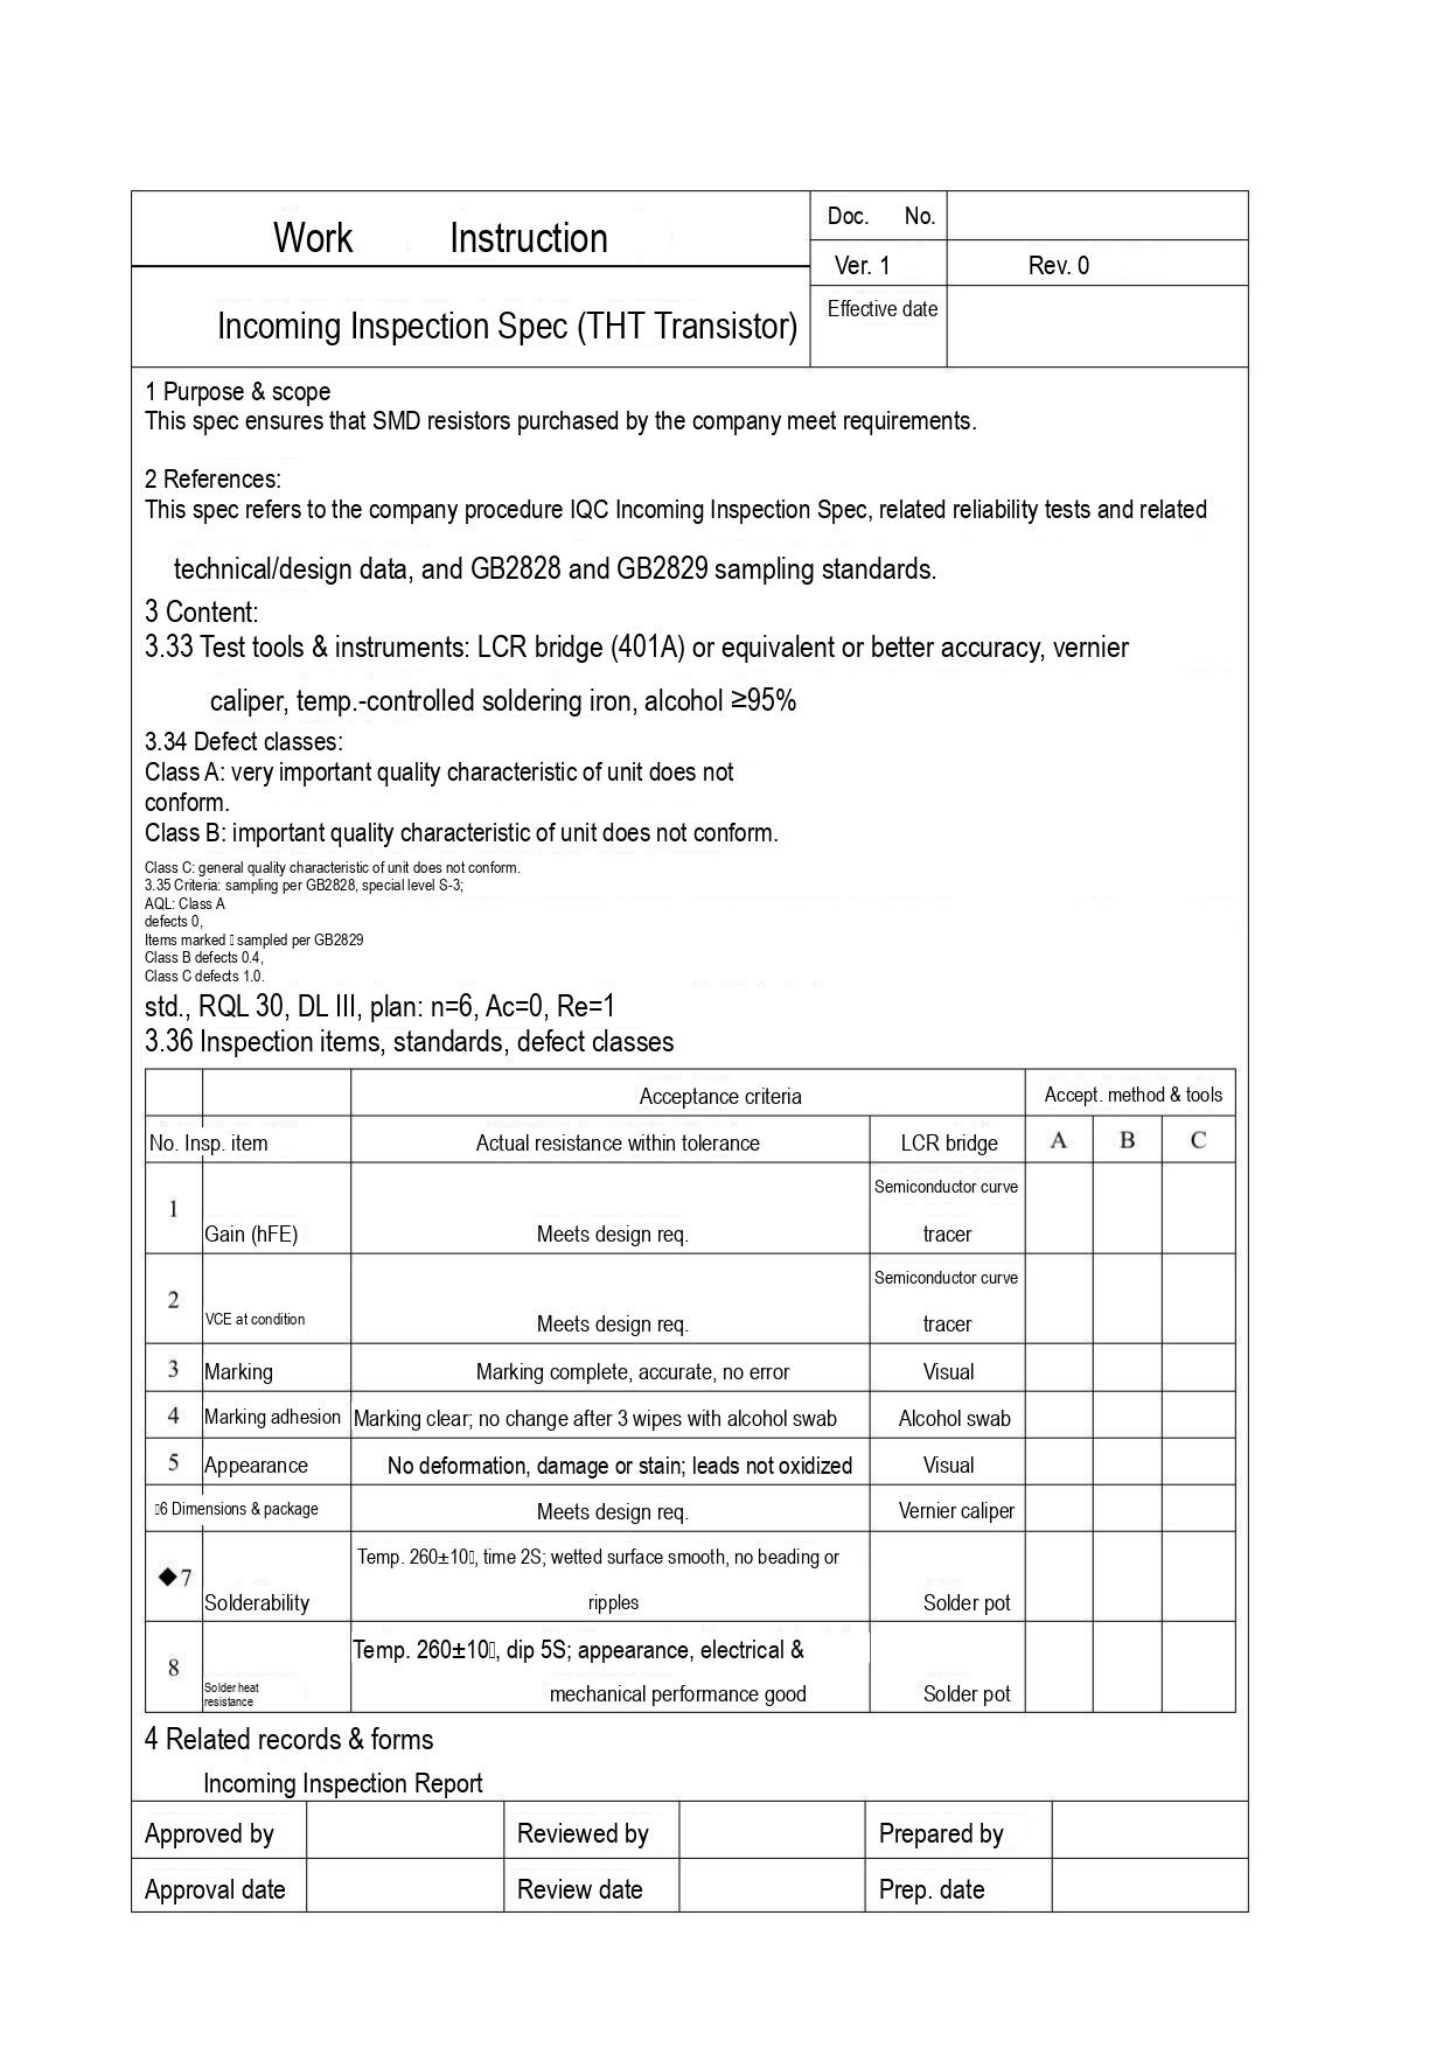| Work Instruction | Doc. No. | |
|---|---|---|
| | Ver. 1 | Rev. 0 |
| Incoming Inspection Spec (THT Transistor) | Effective date | |

1 Purpose & scope
This spec ensures that SMD resistors purchased by the company meet requirements.

2 References:
This spec refers to the company procedure IQC Incoming Inspection Spec, related reliability tests and related technical/design data, and GB2828 and GB2829 sampling standards.

3 Content:
3.33 Test tools & instruments: LCR bridge (401A) or equivalent or better accuracy, vernier caliper, temp.-controlled soldering iron, alcohol ≥95%
3.34 Defect classes:
Class A: very important quality characteristic of unit does not conform.
Class B: important quality characteristic of unit does not conform.
Class C: general quality characteristic of unit does not conform.
3.35 Criteria: sampling per GB2828, special level S-3;
AQL: Class A
defects 0,
Items marked □ sampled per GB2829
Class B defects 0.4,
Class C defects 1.0.
std., RQL 30, DL III, plan: n=6, Ac=0, Re=1
3.36 Inspection items, standards, defect classes

| | | Acceptance criteria | | Accept. method & tools | | |
|---|---|---|---|---|---|---|
| No. | Insp. item | Actual resistance within tolerance | LCR bridge | A | B | C |
| 1 | Gain (hFE) | Meets design req. | Semiconductor curve tracer | | | |
| 2 | VCE at condition | Meets design req. | Semiconductor curve tracer | | | |
| 3 | Marking | Marking complete, accurate, no error | Visual | | | |
| 4 | Marking adhesion | Marking clear; no change after 3 wipes with alcohol swab | Alcohol swab | | | |
| 5 | Appearance | No deformation, damage or stain; leads not oxidized | Visual | | | |
| □6 | Dimensions & package | Meets design req. | Vernier caliper | | | |
| ◆7 | Solderability | Temp. 260±10□, time 2S; wetted surface smooth, no beading or ripples | Solder pot | | | |
| 8 | Solder heat resistance | Temp. 260±10□, dip 5S; appearance, electrical & mechanical performance good | Solder pot | | | |

4 Related records & forms
Incoming Inspection Report

| Approved by | | Reviewed by | | Prepared by | |
|---|---|---|---|---|---|
| Approval date | | Review date | | Prep. date | |
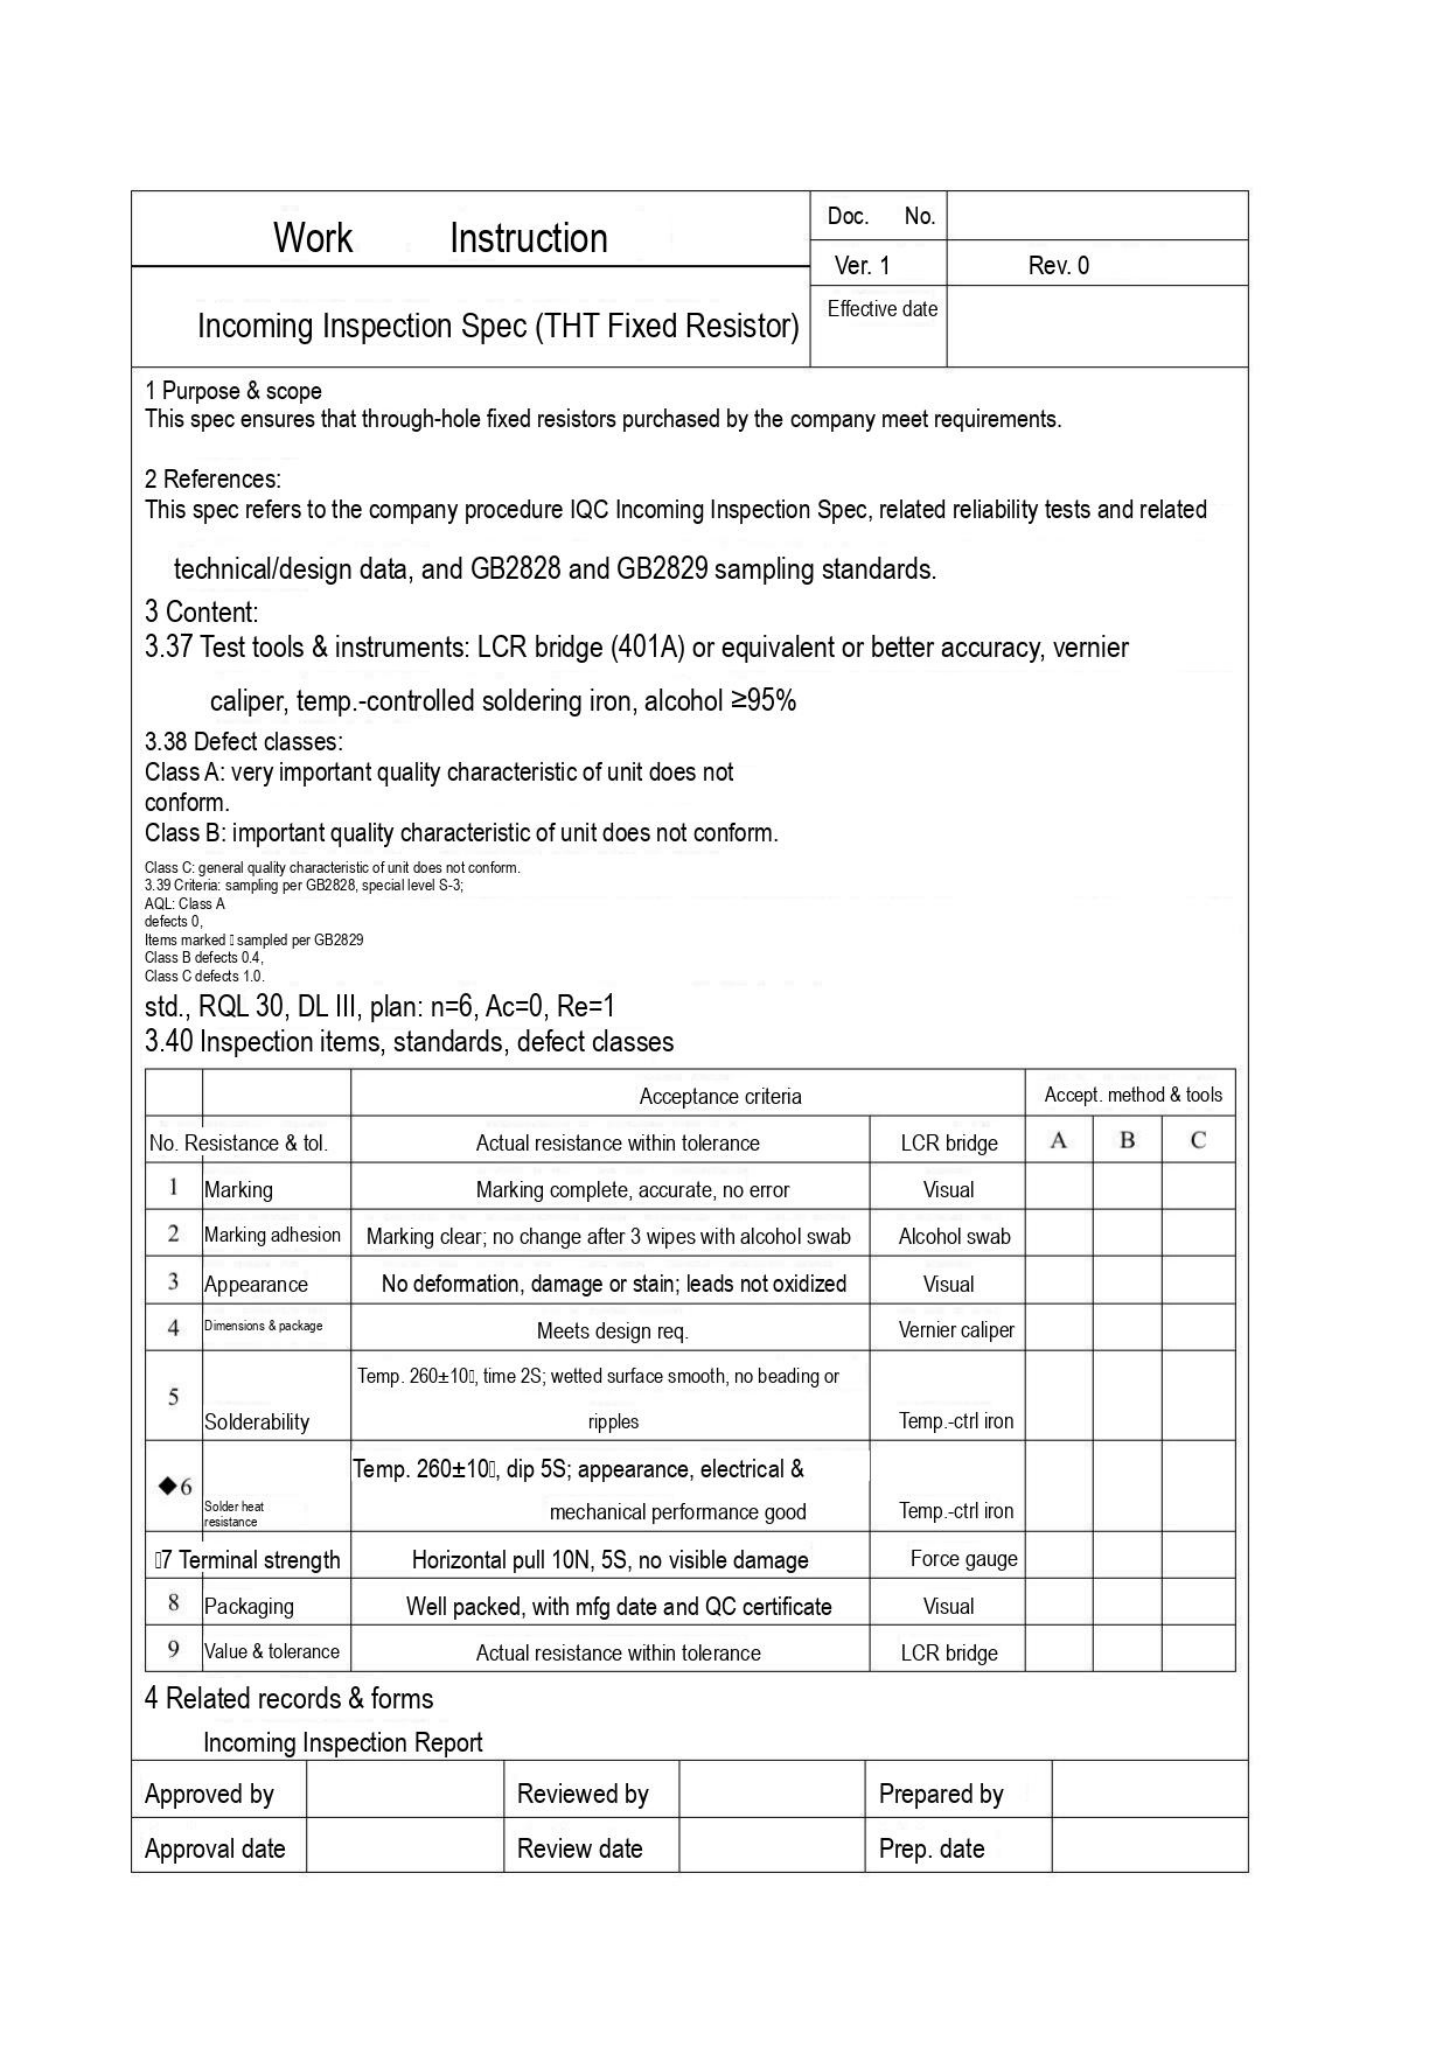| Work Instruction | Doc. No. | |
|---|---|---|
| | Ver. 1 | Rev. 0 |
| Incoming Inspection Spec (THT Fixed Resistor) | Effective date | |

1 Purpose & scope
This spec ensures that through-hole fixed resistors purchased by the company meet requirements.

2 References:
This spec refers to the company procedure IQC Incoming Inspection Spec, related reliability tests and related technical/design data, and GB2828 and GB2829 sampling standards.

3 Content:
3.37 Test tools & instruments: LCR bridge (401A) or equivalent or better accuracy, vernier caliper, temp.-controlled soldering iron, alcohol ≥95%
3.38 Defect classes:
Class A: very important quality characteristic of unit does not conform.
Class B: important quality characteristic of unit does not conform.
Class C: general quality characteristic of unit does not conform.
3.39 Criteria: sampling per GB2828, special level S-3;
AQL: Class A defects 0,
Items marked □ sampled per GB2829
Class B defects 0.4,
Class C defects 1.0.
std., RQL 30, DL III, plan: n=6, Ac=0, Re=1
3.40 Inspection items, standards, defect classes

| | | Acceptance criteria | | Accept. method & tools | | |
|---|---|---|---|---|---|---|
| No. | Resistance & tol. | Actual resistance within tolerance | LCR bridge | A | B | C |
| 1 | Marking | Marking complete, accurate, no error | Visual | | | |
| 2 | Marking adhesion | Marking clear; no change after 3 wipes with alcohol swab | Alcohol swab | | | |
| 3 | Appearance | No deformation, damage or stain; leads not oxidized | Visual | | | |
| 4 | Dimensions & package | Meets design req. | Vernier caliper | | | |
| 5 | Solderability | Temp. 260±10□, time 2S; wetted surface smooth, no beading or ripples | Temp.-ctrl iron | | | |
| ◆6 | Solder heat resistance | Temp. 260±10□, dip 5S; appearance, electrical & mechanical performance good | Temp.-ctrl iron | | | |
| □7 | Terminal strength | Horizontal pull 10N, 5S, no visible damage | Force gauge | | | |
| 8 | Packaging | Well packed, with mfg date and QC certificate | Visual | | | |
| 9 | Value & tolerance | Actual resistance within tolerance | LCR bridge | | | |

4 Related records & forms
Incoming Inspection Report

| Approved by | | Reviewed by | | Prepared by | |
|---|---|---|---|---|---|
| Approval date | | Review date | | Prep. date | |
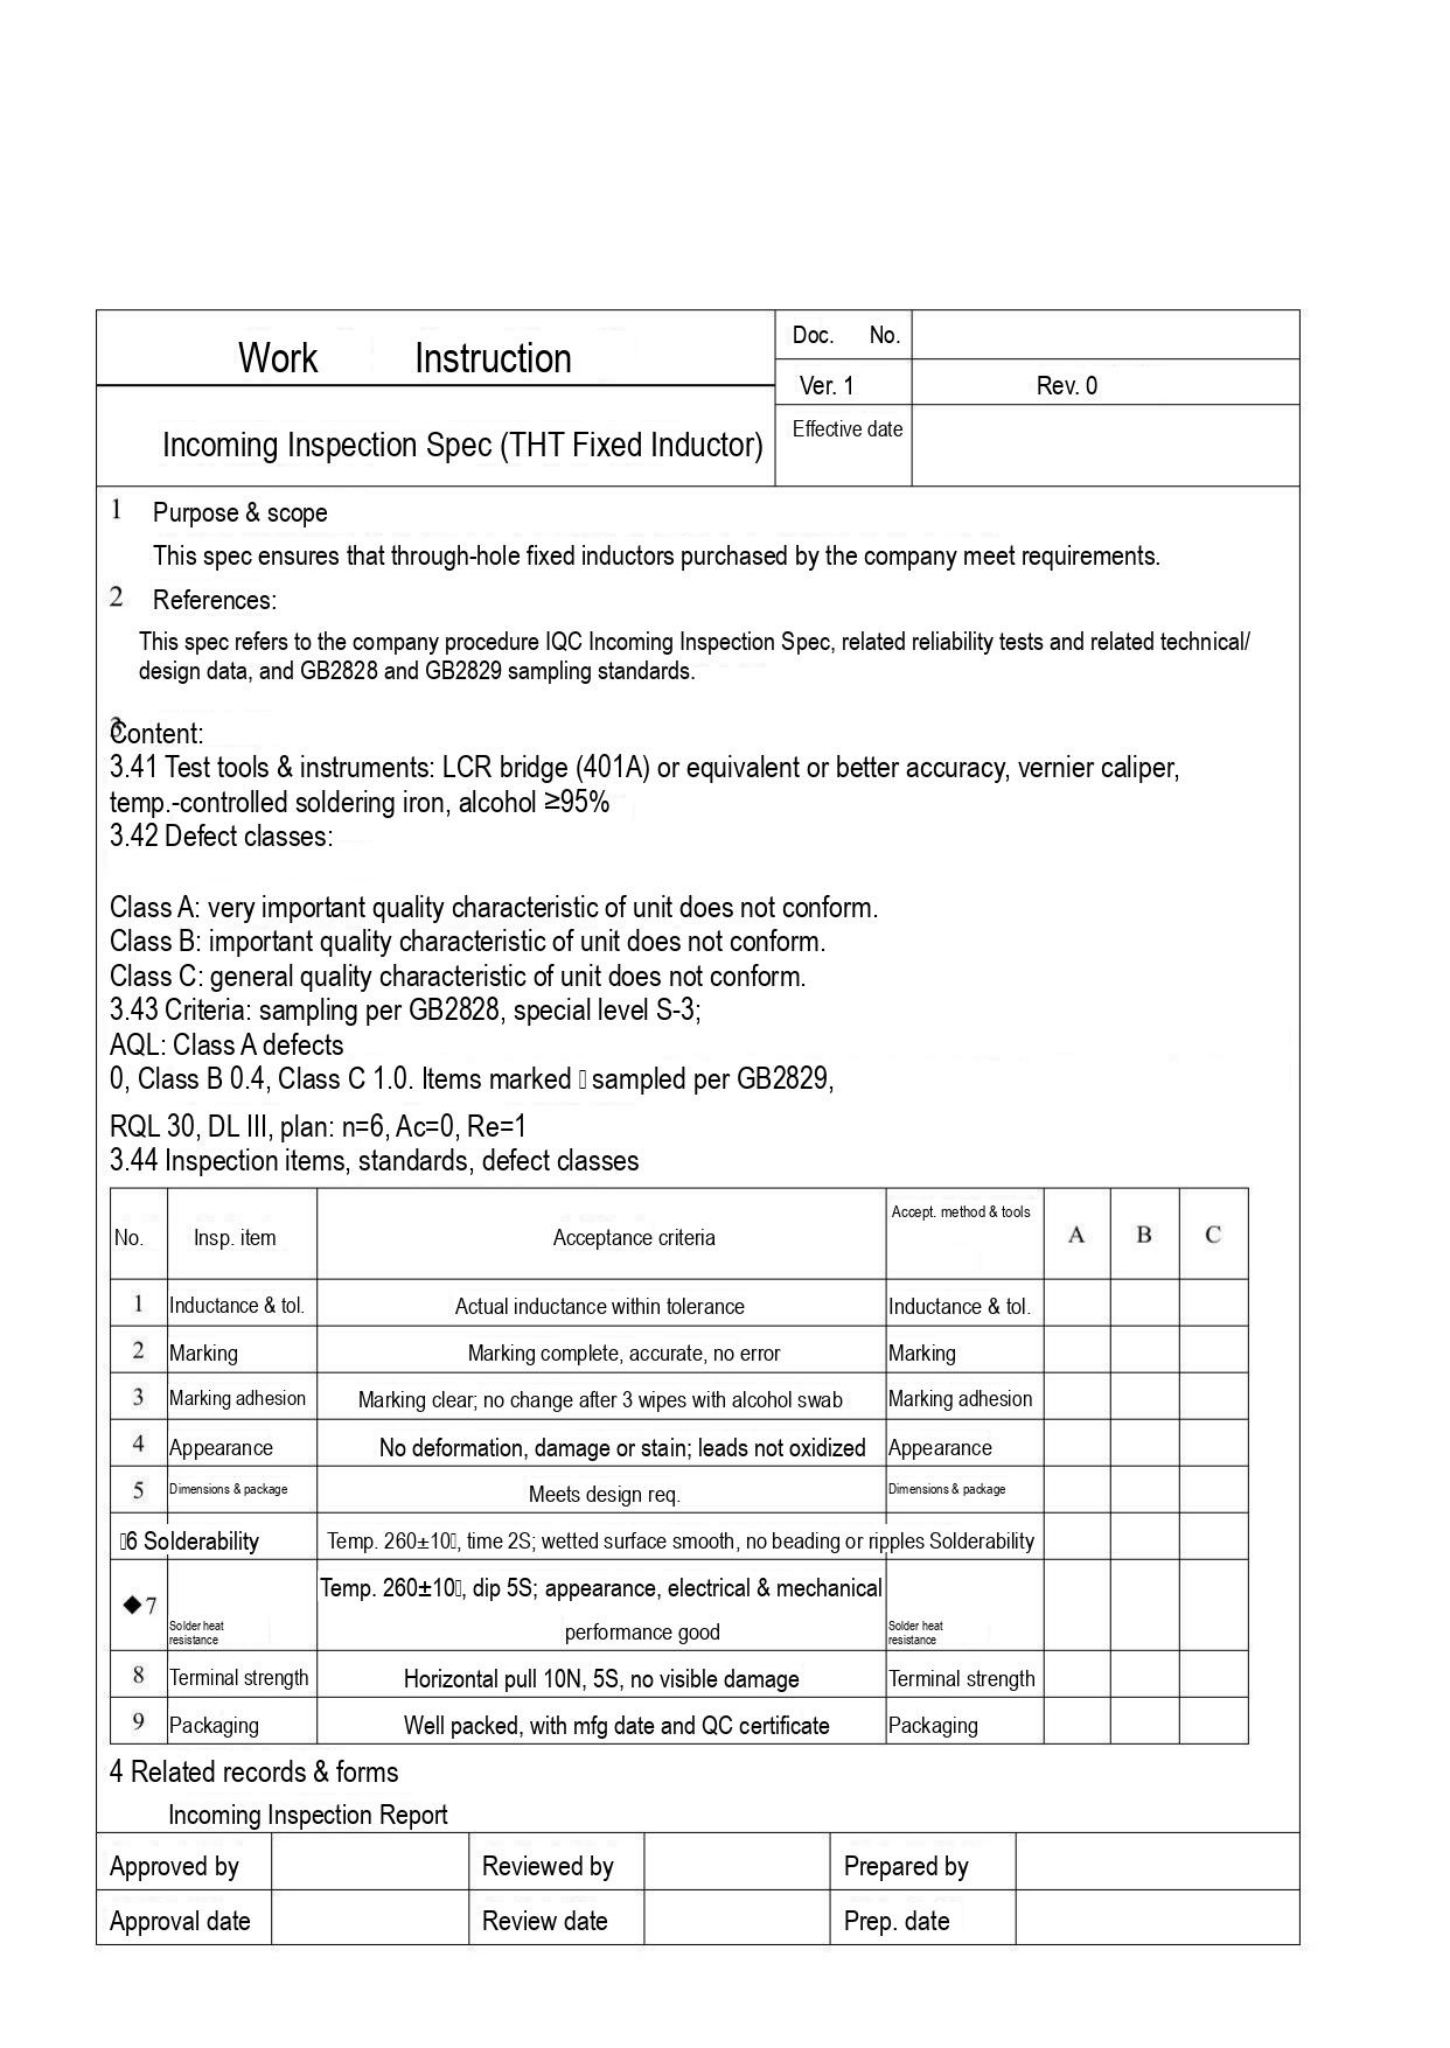# Work Instruction

| Work Instruction | Doc. No. | |
|---|---|---|
| | Ver. 1 | Rev. 0 |
| Incoming Inspection Spec (THT Fixed Inductor) | Effective date | |

1 Purpose & scope

This spec ensures that through-hole fixed inductors purchased by the company meet requirements.

2 References:

This spec refers to the company procedure IQC Incoming Inspection Spec, related reliability tests and related technical/ design data, and GB2828 and GB2829 sampling standards.

3 Content:

3.41 Test tools & instruments: LCR bridge (401A) or equivalent or better accuracy, vernier caliper, temp.-controlled soldering iron, alcohol ≥95%

3.42 Defect classes:

Class A: very important quality characteristic of unit does not conform.
Class B: important quality characteristic of unit does not conform.
Class C: general quality characteristic of unit does not conform.

3.43 Criteria: sampling per GB2828, special level S-3;
AQL: Class A defects
0, Class B 0.4, Class C 1.0. Items marked □ sampled per GB2829,

RQL 30, DL III, plan: n=6, Ac=0, Re=1

3.44 Inspection items, standards, defect classes

| No. | Insp. item | Acceptance criteria | Accept. method & tools | A | B | C |
|---|---|---|---|---|---|---|
| 1 | Inductance & tol. | Actual inductance within tolerance | Inductance & tol. | | | |
| 2 | Marking | Marking complete, accurate, no error | Marking | | | |
| 3 | Marking adhesion | Marking clear; no change after 3 wipes with alcohol swab | Marking adhesion | | | |
| 4 | Appearance | No deformation, damage or stain; leads not oxidized | Appearance | | | |
| 5 | Dimensions & package | Meets design req. | Dimensions & package | | | |
| □6 | Solderability | Temp. 260±10□, time 2S; wetted surface smooth, no beading or ripples | Solderability | | | |
| ◆7 | Solder heat resistance | Temp. 260±10□, dip 5S; appearance, electrical & mechanical performance good | Solder heat resistance | | | |
| 8 | Terminal strength | Horizontal pull 10N, 5S, no visible damage | Terminal strength | | | |
| 9 | Packaging | Well packed, with mfg date and QC certificate | Packaging | | | |

4 Related records & forms

Incoming Inspection Report

| Approved by | | Reviewed by | | Prepared by | |
|---|---|---|---|---|---|
| Approval date | | Review date | | Prep. date | |
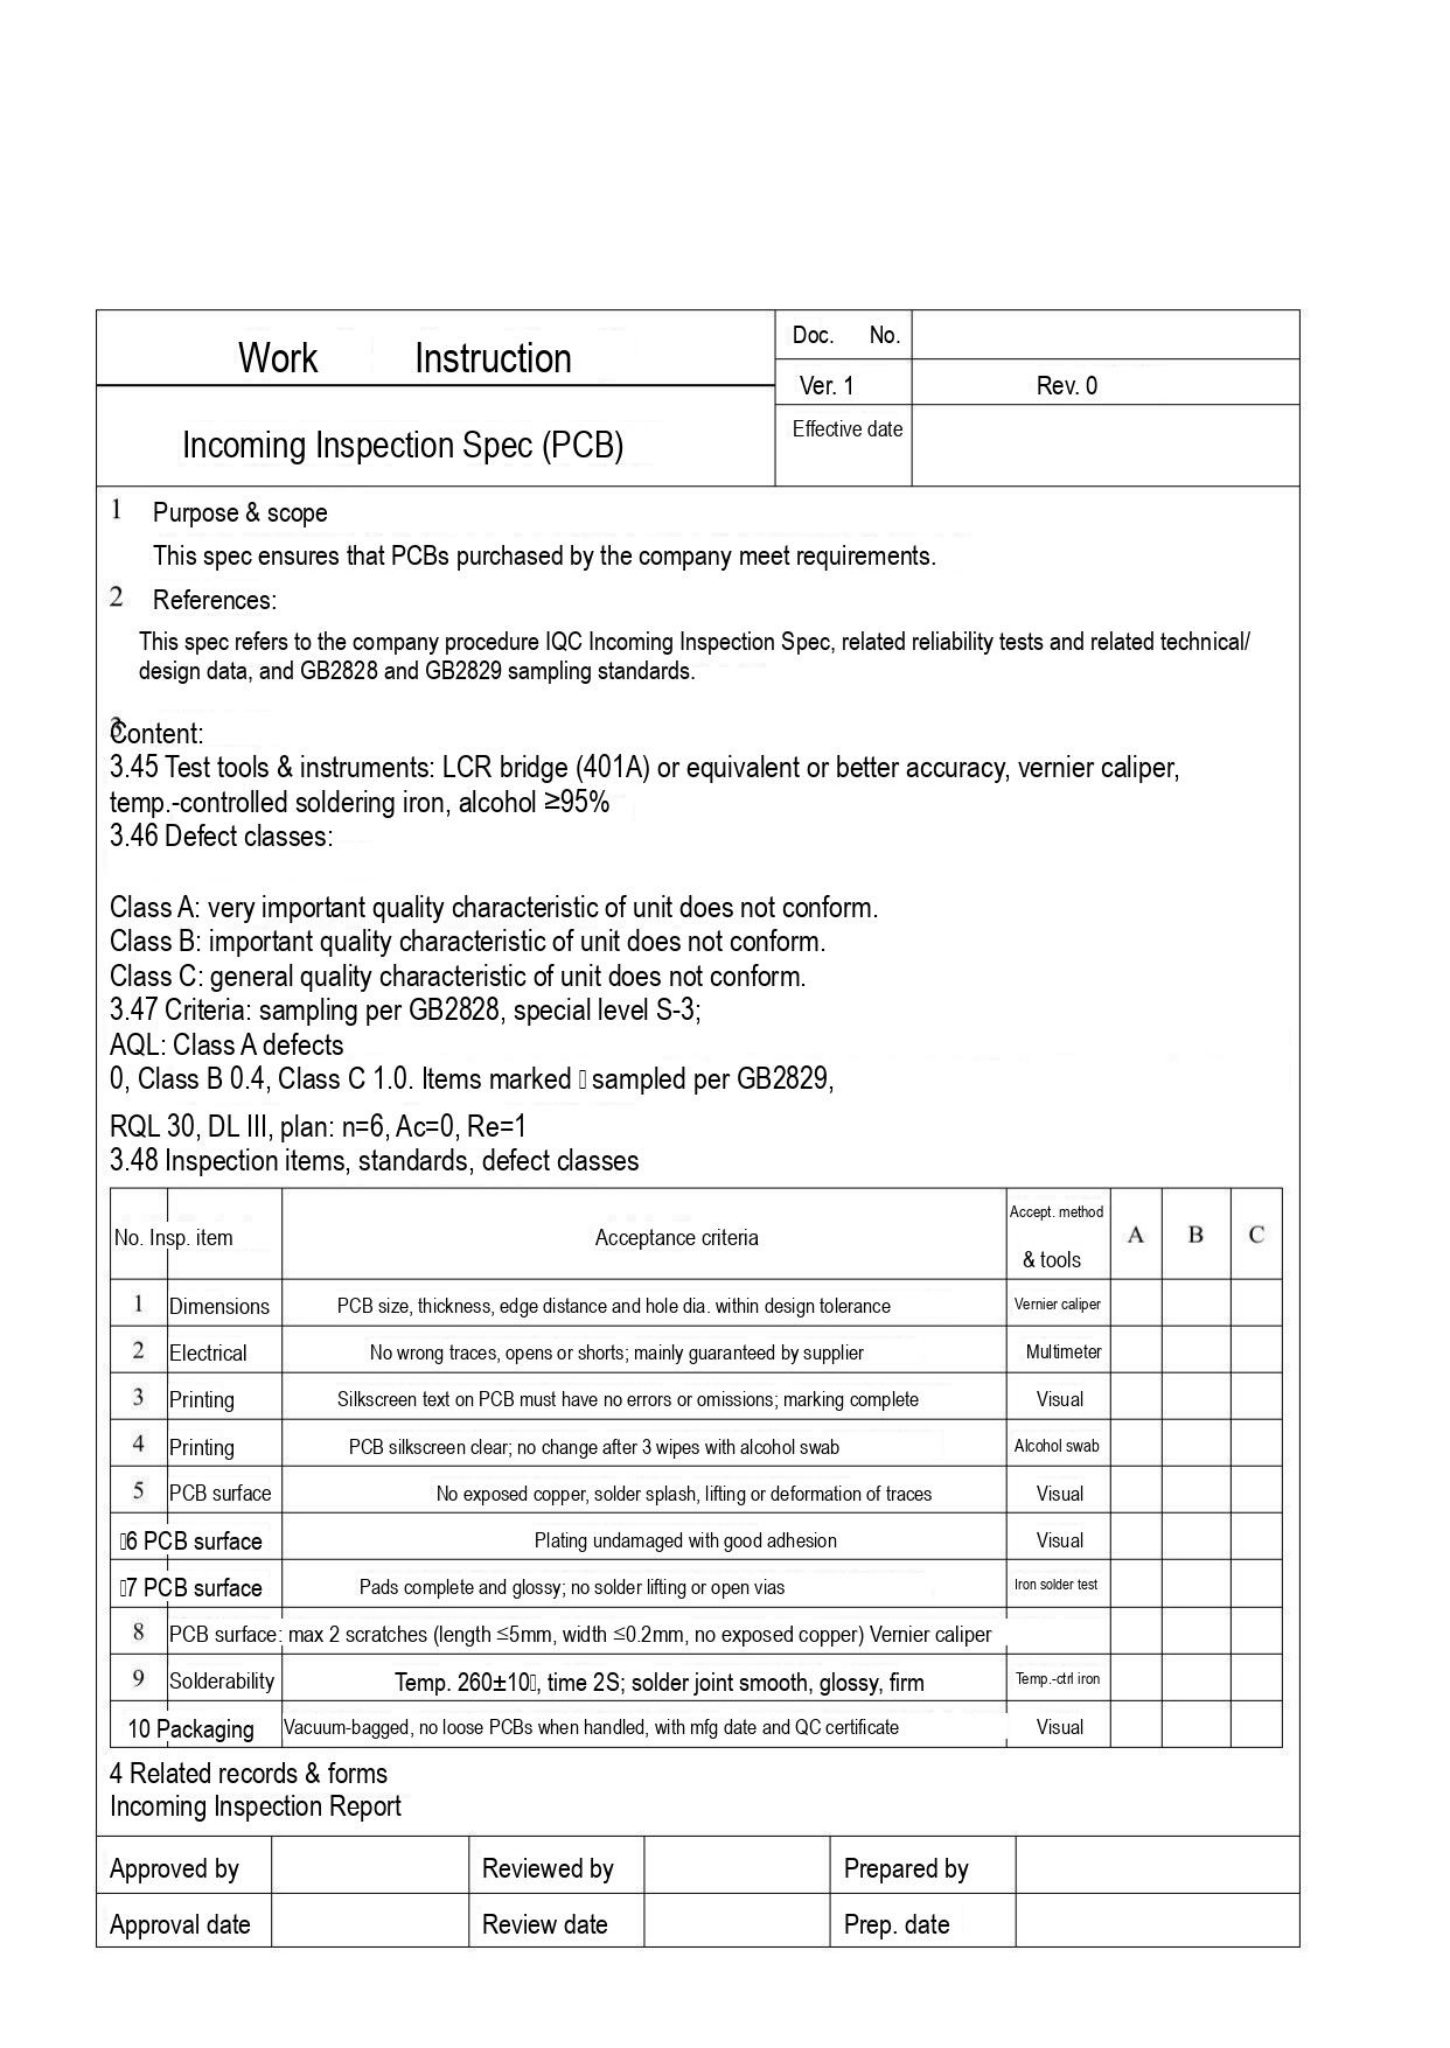# Work Instruction

| Doc. No. | |
|---|---|
| Ver. 1 | Rev. 0 |
| Effective date | |

Incoming Inspection Spec (PCB)

1 Purpose & scope

This spec ensures that PCBs purchased by the company meet requirements.

2 References:

This spec refers to the company procedure IQC Incoming Inspection Spec, related reliability tests and related technical/design data, and GB2828 and GB2829 sampling standards.

3 Content:

3.45 Test tools & instruments: LCR bridge (401A) or equivalent or better accuracy, vernier caliper, temp.-controlled soldering iron, alcohol ≥95%

3.46 Defect classes:

Class A: very important quality characteristic of unit does not conform.
Class B: important quality characteristic of unit does not conform.
Class C: general quality characteristic of unit does not conform.

3.47 Criteria: sampling per GB2828, special level S-3;
AQL: Class A defects
0, Class B 0.4, Class C 1.0. Items marked sampled per GB2829,

RQL 30, DL III, plan: n=6, Ac=0, Re=1

3.48 Inspection items, standards, defect classes

| No. | Insp. item | Acceptance criteria | Accept. method & tools | A | B | C |
|---|---|---|---|---|---|---|
| 1 | Dimensions | PCB size, thickness, edge distance and hole dia. within design tolerance | Vernier caliper | | | |
| 2 | Electrical | No wrong traces, opens or shorts; mainly guaranteed by supplier | Multimeter | | | |
| 3 | Printing | Silkscreen text on PCB must have no errors or omissions; marking complete | Visual | | | |
| 4 | Printing | PCB silkscreen clear; no change after 3 wipes with alcohol swab | Alcohol swab | | | |
| 5 | PCB surface | No exposed copper, solder splash, lifting or deformation of traces | Visual | | | |
| 6 | PCB surface | Plating undamaged with good adhesion | Visual | | | |
| 7 | PCB surface | Pads complete and glossy; no solder lifting or open vias | Iron solder test | | | |
| 8 | PCB surface: | max 2 scratches (length ≤5mm, width ≤0.2mm, no exposed copper) | Vernier caliper | | | |
| 9 | Solderability | Temp. 260±10, time 2S; solder joint smooth, glossy, firm | Temp.-ctrl iron | | | |
| 10 | Packaging | Vacuum-bagged, no loose PCBs when handled, with mfg date and QC certificate | Visual | | | |

4 Related records & forms
Incoming Inspection Report

| Approved by | | Reviewed by | | Prepared by | |
|---|---|---|---|---|---|
| Approval date | | Review date | | Prep. date | |
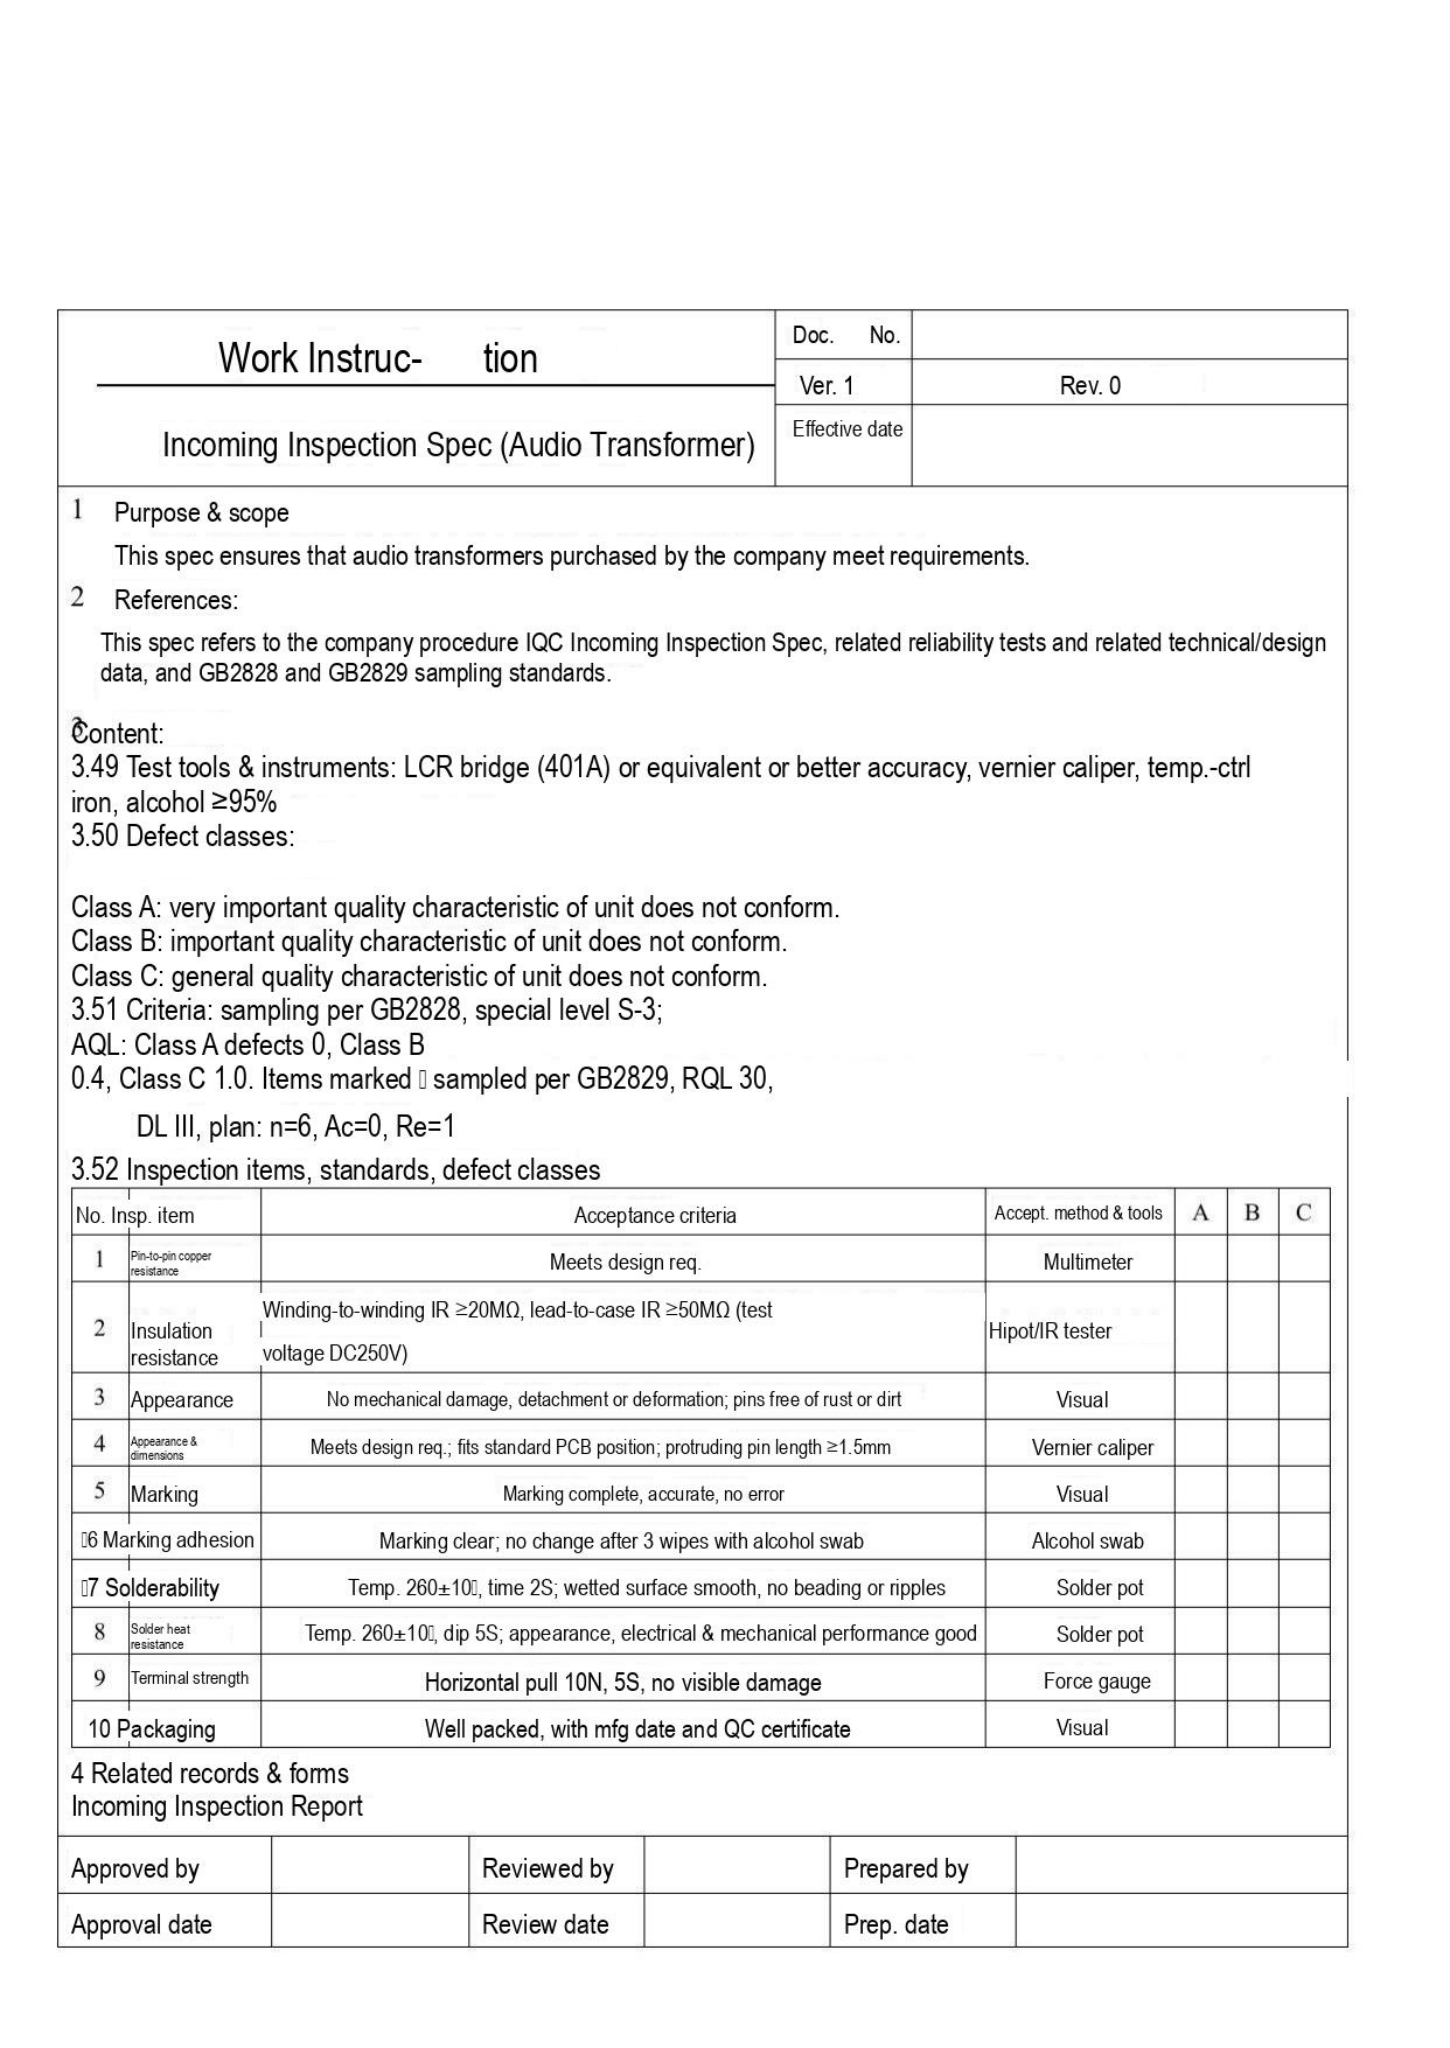| Work Instruc- tion | Doc. No. | |
|---|---|---|
| | Ver. 1 | Rev. 0 |
| Incoming Inspection Spec (Audio Transformer) | Effective date | |

1 Purpose & scope

This spec ensures that audio transformers purchased by the company meet requirements.

2 References:

This spec refers to the company procedure IQC Incoming Inspection Spec, related reliability tests and related technical/design data, and GB2828 and GB2829 sampling standards.

3 Content:

3.49 Test tools & instruments: LCR bridge (401A) or equivalent or better accuracy, vernier caliper, temp.-ctrl iron, alcohol ≥95%

3.50 Defect classes:

Class A: very important quality characteristic of unit does not conform.
Class B: important quality characteristic of unit does not conform.
Class C: general quality characteristic of unit does not conform.

3.51 Criteria: sampling per GB2828, special level S-3;
AQL: Class A defects 0, Class B
0.4, Class C 1.0. Items marked sampled per GB2829, RQL 30,
DL III, plan: n=6, Ac=0, Re=1

3.52 Inspection items, standards, defect classes

| No. | Insp. item | Acceptance criteria | Accept. method & tools | A | B | C |
|---|---|---|---|---|---|---|
| 1 | Pin-to-pin copper resistance | Meets design req. | Multimeter | | | |
| 2 | Insulation resistance | Winding-to-winding IR ≥20MΩ, lead-to-case IR ≥50MΩ (test voltage DC250V) | Hipot/IR tester | | | |
| 3 | Appearance | No mechanical damage, detachment or deformation; pins free of rust or dirt | Visual | | | |
| 4 | Appearance & dimensions | Meets design req.; fits standard PCB position; protruding pin length ≥1.5mm | Vernier caliper | | | |
| 5 | Marking | Marking complete, accurate, no error | Visual | | | |
| 6 | Marking adhesion | Marking clear; no change after 3 wipes with alcohol swab | Alcohol swab | | | |
| 7 | Solderability | Temp. 260±10, time 2S; wetted surface smooth, no beading or ripples | Solder pot | | | |
| 8 | Solder heat resistance | Temp. 260±10, dip 5S; appearance, electrical & mechanical performance good | Solder pot | | | |
| 9 | Terminal strength | Horizontal pull 10N, 5S, no visible damage | Force gauge | | | |
| 10 | Packaging | Well packed, with mfg date and QC certificate | Visual | | | |

4 Related records & forms
Incoming Inspection Report

| Approved by | | Reviewed by | | Prepared by | |
|---|---|---|---|---|---|
| Approval date | | Review date | | Prep. date | |
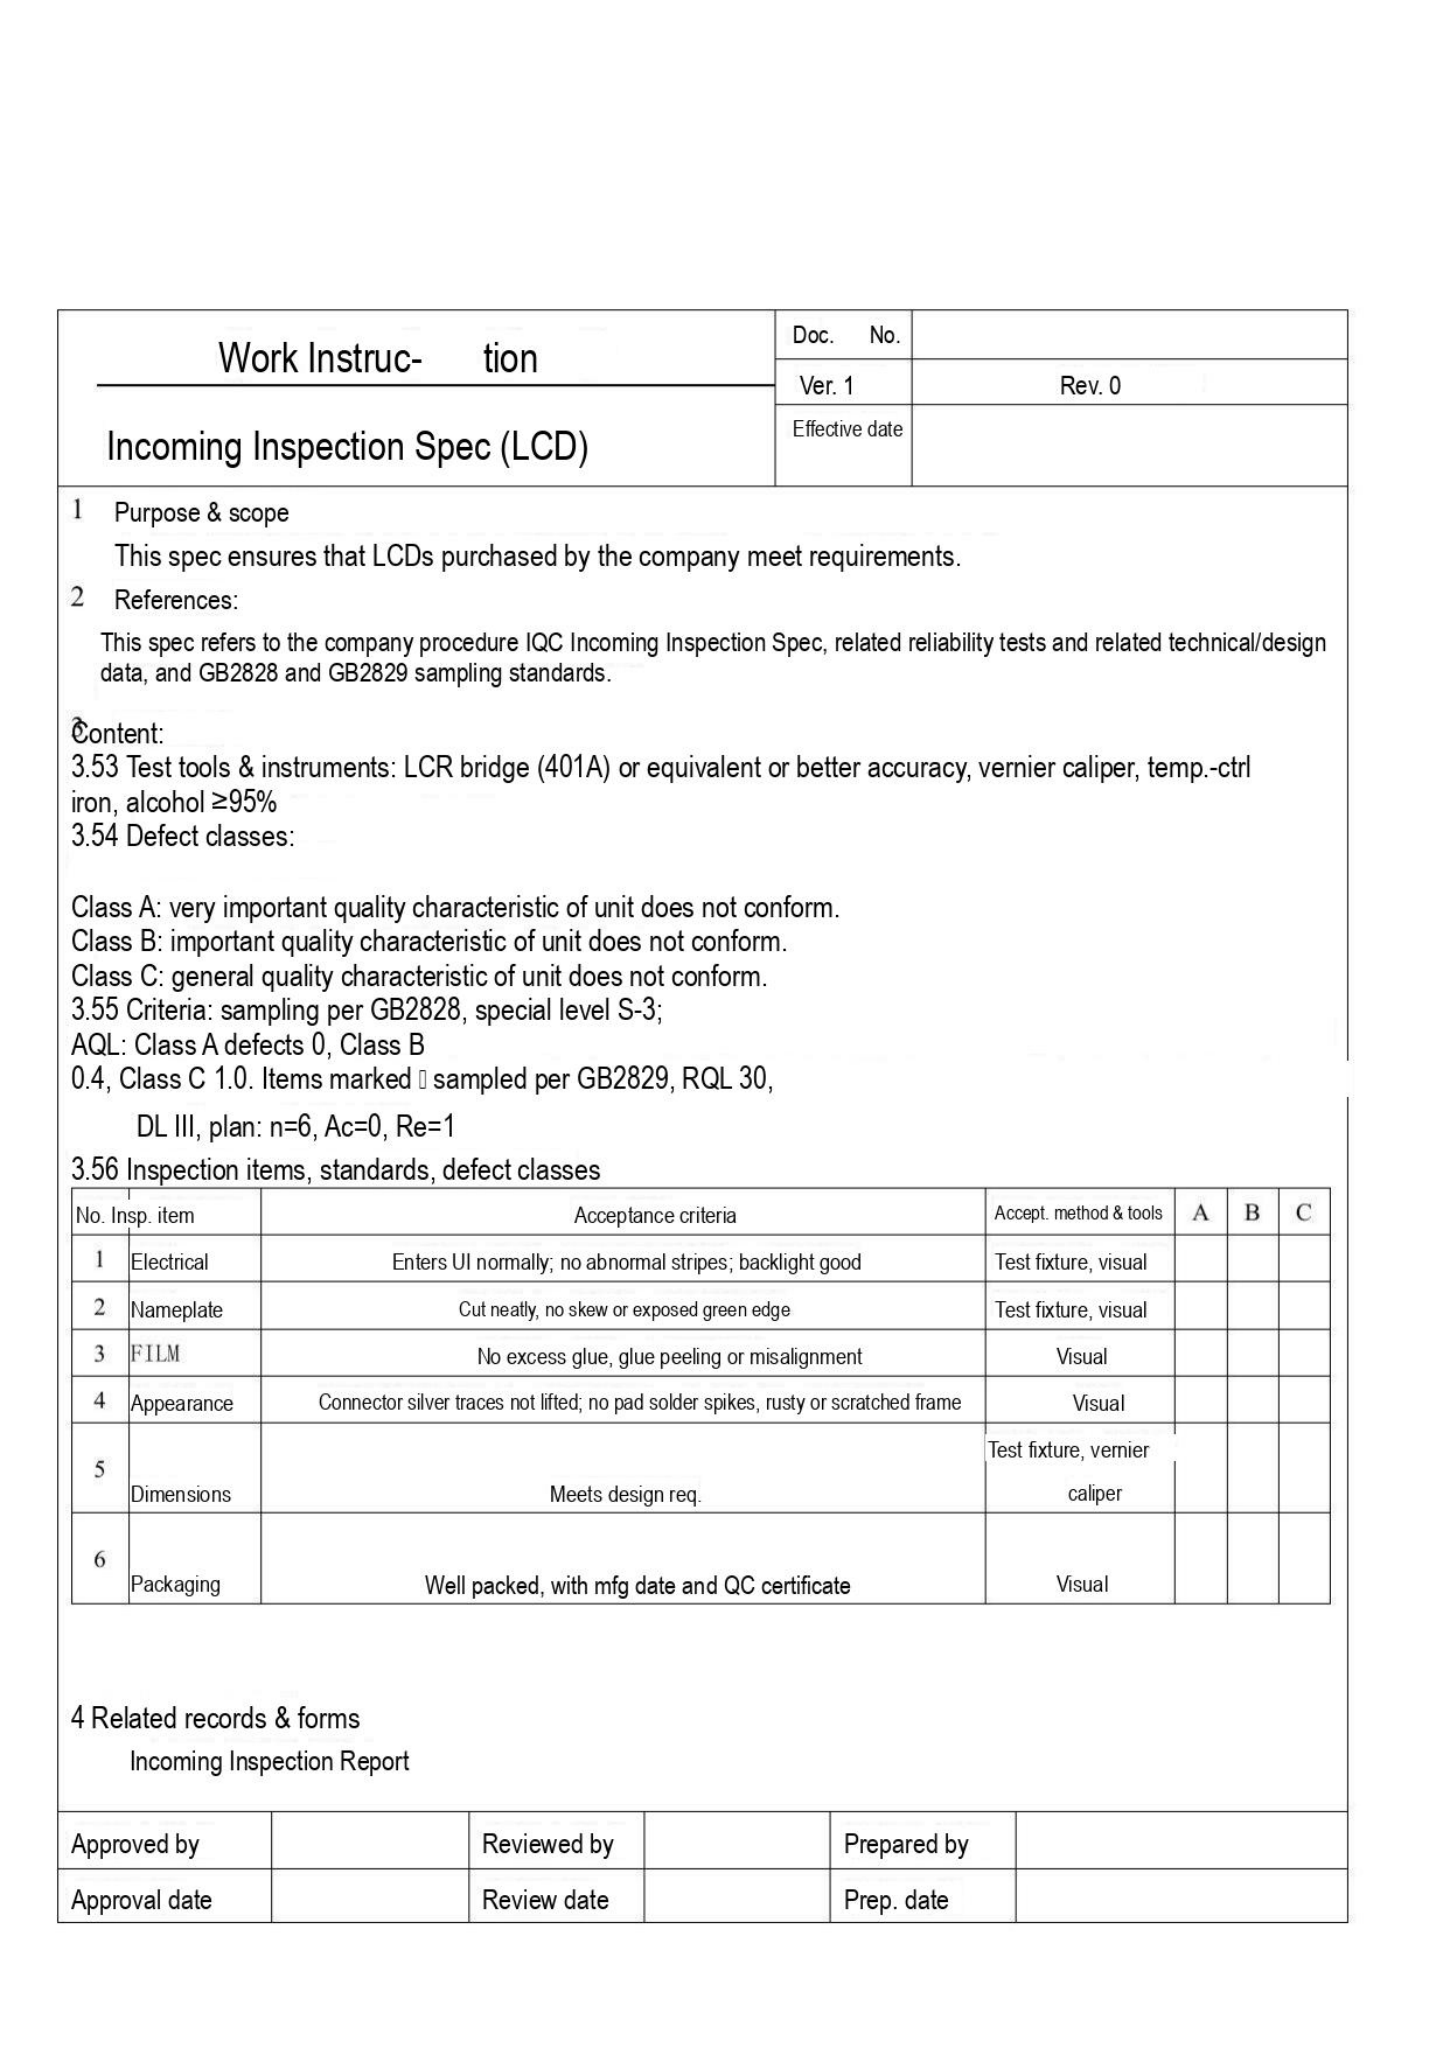| Work Instruc- tion | Doc. No. | |
|---|---|---|
| | Ver. 1 | Rev. 0 |
| Incoming Inspection Spec (LCD) | Effective date | |

1 Purpose & scope

This spec ensures that LCDs purchased by the company meet requirements.

2 References:

This spec refers to the company procedure IQC Incoming Inspection Spec, related reliability tests and related technical/design data, and GB2828 and GB2829 sampling standards.

3 Content:

3.53 Test tools & instruments: LCR bridge (401A) or equivalent or better accuracy, vernier caliper, temp.-ctrl iron, alcohol ≥95%

3.54 Defect classes:

Class A: very important quality characteristic of unit does not conform.
Class B: important quality characteristic of unit does not conform.
Class C: general quality characteristic of unit does not conform.

3.55 Criteria: sampling per GB2828, special level S-3;
AQL: Class A defects 0, Class B
0.4, Class C 1.0. Items marked sampled per GB2829, RQL 30,

DL III, plan: n=6, Ac=0, Re=1

3.56 Inspection items, standards, defect classes

| No. | Insp. item | Acceptance criteria | Accept. method & tools | A | B | C |
|---|---|---|---|---|---|---|
| 1 | Electrical | Enters UI normally; no abnormal stripes; backlight good | Test fixture, visual | | | |
| 2 | Nameplate | Cut neatly, no skew or exposed green edge | Test fixture, visual | | | |
| 3 | FILM | No excess glue, glue peeling or misalignment | Visual | | | |
| 4 | Appearance | Connector silver traces not lifted; no pad solder spikes, rusty or scratched frame | Visual | | | |
| 5 | Dimensions | Meets design req. | Test fixture, vernier caliper | | | |
| 6 | Packaging | Well packed, with mfg date and QC certificate | Visual | | | |

4 Related records & forms

Incoming Inspection Report

| Approved by | | Reviewed by | | Prepared by | |
|---|---|---|---|---|---|
| Approval date | | Review date | | Prep. date | |